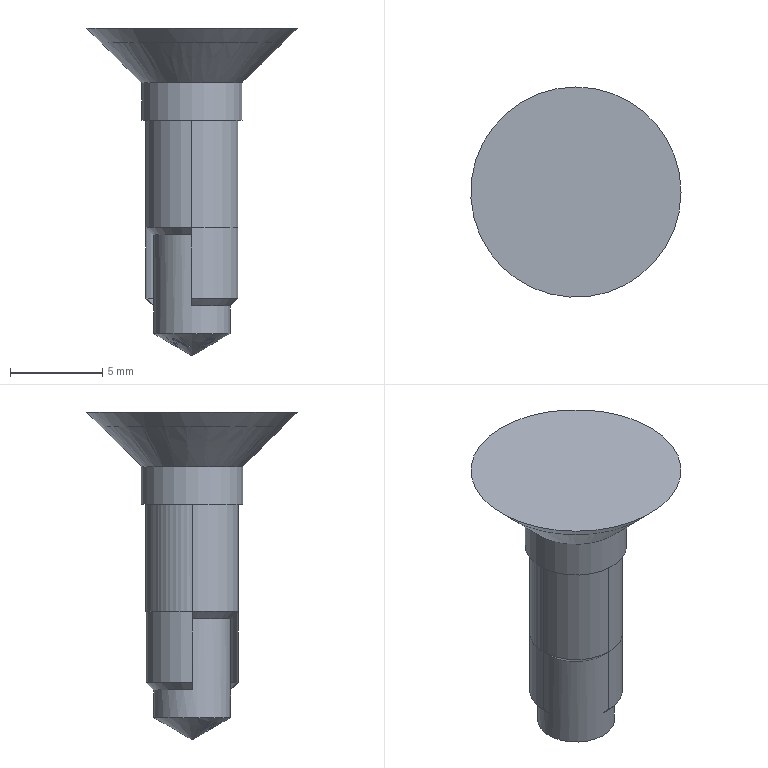Part | STEP file | EM40500800 | 3 solids | 79 faces | box 11.4 x 11.4 x 17.76 mm | volume 658.01 mm3 | plane 55 | other 10 | cone 8 | cylinder 6 | commonest cylinder face diameters 5 x2 4.167 x1 4.983 x1 5.5 x1 9.8 x1